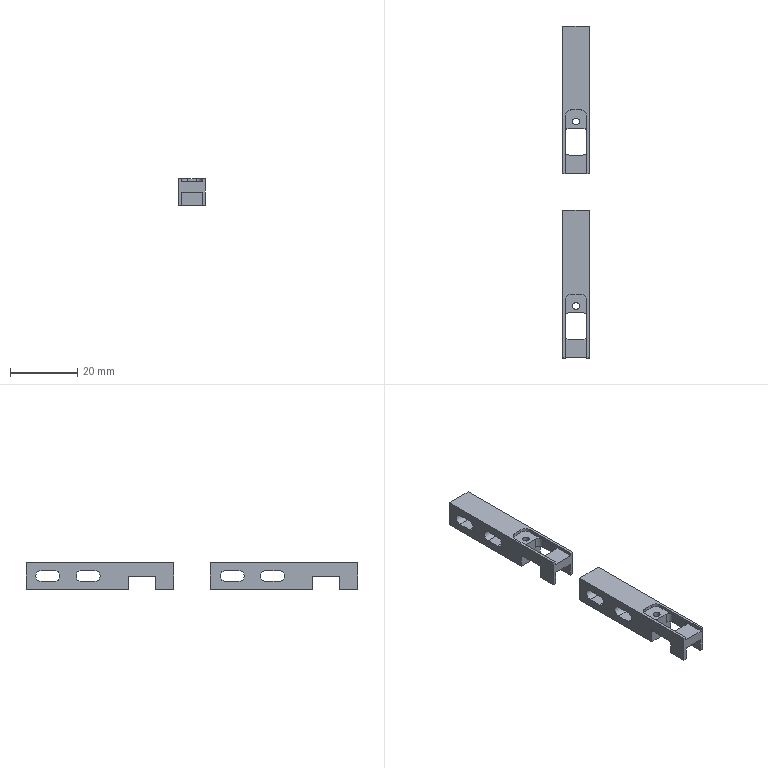Part | 2 solids | 98 faces | box 8 x 99 x 8 mm | volume 3198 mm3 | plane 68 | cylinder 30 | commonest cylinder face diameters 3 x8 3.2 x8 6 x8 4 x4 2.05 x2